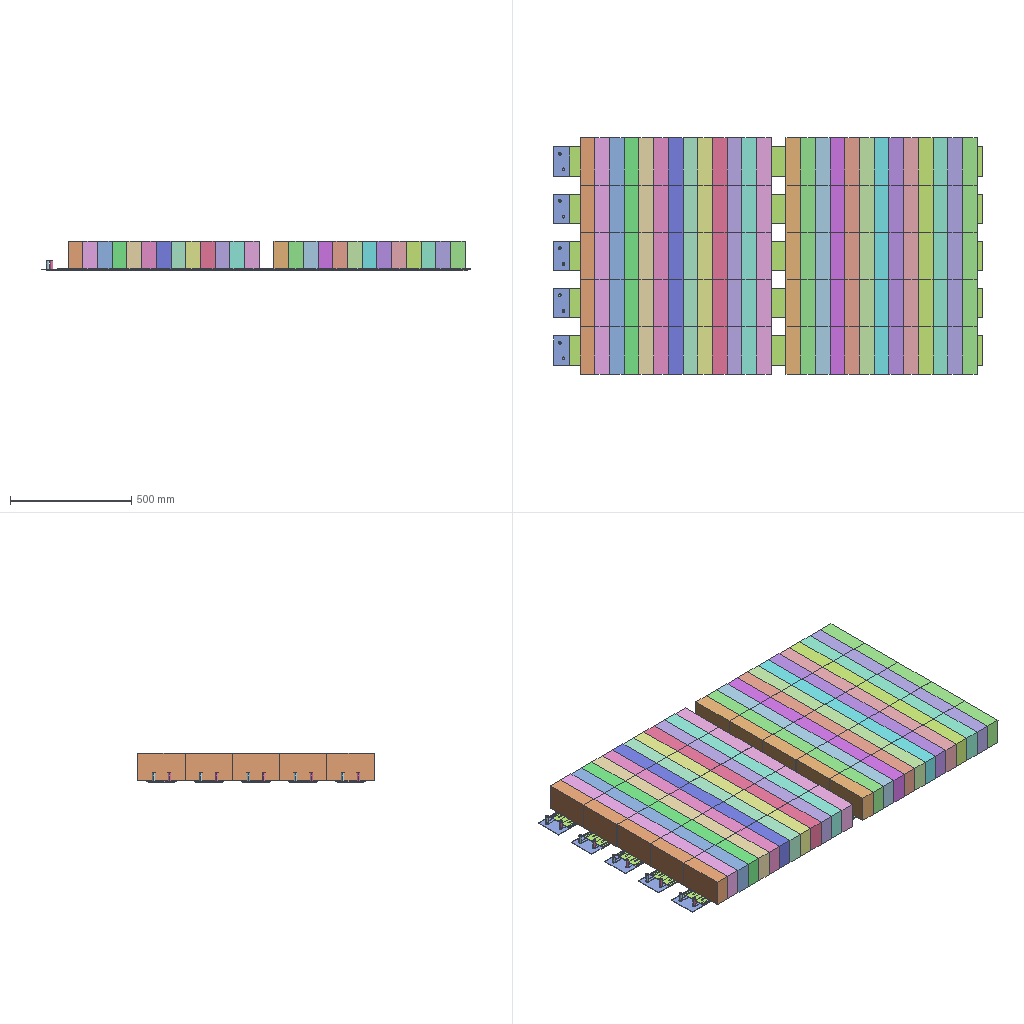Assembly | SolidWorks | 32 different items | 160 placed | box 1768 x 975 x 120 mm
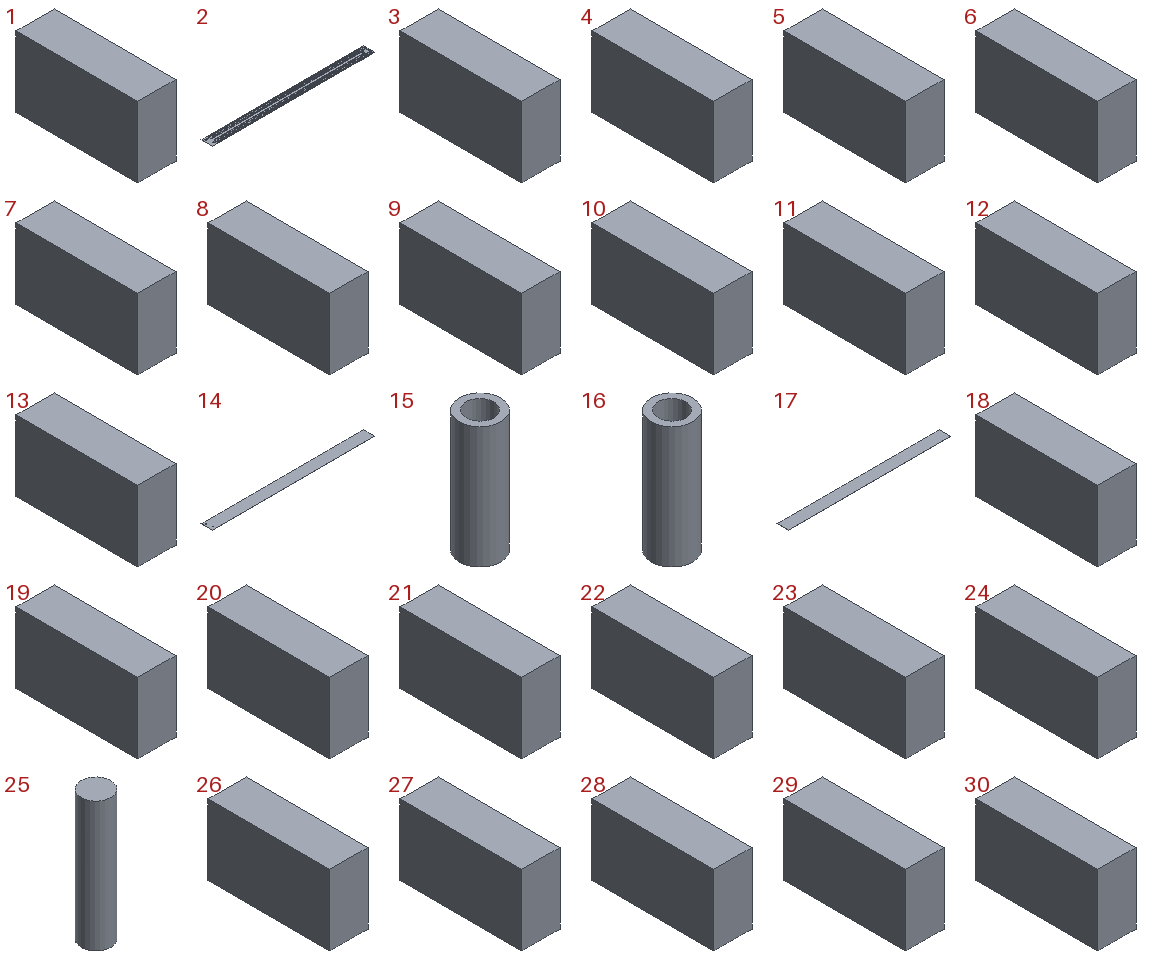Parts list (item | quantity | size | volume | features):
1 | x5 | 60.7 x 194.65 x 112.8 mm | 1332761 mm3 | features BaseBody 1
2 | x5 | 1768 x 120 x 5 mm | 357777 mm3 | features ICE 4, BaseBody 1, LPattern 1
3 | x5 | 60.7 x 194.65 x 112.8 mm | 1332761 mm3 | features BaseBody 1
4 | x5 | 60.7 x 194.65 x 112.8 mm | 1332761 mm3 | features BaseBody 1
5 | x5 | 60.7 x 194.65 x 112.8 mm | 1332761 mm3 | features BaseBody 1
6 | x5 | 60.7 x 194.65 x 112.8 mm | 1332761 mm3 | features BaseBody 1
7 | x5 | 60.7 x 194.65 x 112.8 mm | 1332761 mm3 | features BaseBody 1
8 | x5 | 60.7 x 194.65 x 112.8 mm | 1332761 mm3 | features BaseBody 1
9 | x5 | 60.7 x 194.65 x 112.8 mm | 1332761 mm3 | features BaseBody 1
10 | x5 | 60.7 x 194.65 x 112.8 mm | 1332761 mm3 | features BaseBody 1
11 | x5 | 60.7 x 194.65 x 112.8 mm | 1332761 mm3 | features BaseBody 1
12 | x5 | 60.7 x 194.65 x 112.8 mm | 1332761 mm3 | features BaseBody 1
13 | x5 | 60.7 x 194.65 x 112.8 mm | 1332761 mm3 | features BaseBody 1
14 | x5 | 1768 x 120 x 1 mm | 211934 mm3 | features BaseBody 1
15 | x5 | 12 x 12 x 35 mm | 2199 mm3 | features BaseBody 1
16 | x5 | 12 x 12 x 35 mm | 2199 mm3 | features BaseBody 1
17 | x5 | 1703 x 120 x 1 mm | 204360 mm3 | features BaseBody 1
18 | x5 | 60.7 x 194.65 x 112.8 mm | 1332761 mm3 | features BaseBody 1
19 | x5 | 60.7 x 194.65 x 112.8 mm | 1332761 mm3 | features BaseBody 1
20 | x5 | 60.7 x 194.65 x 112.8 mm | 1332761 mm3 | features BaseBody 1
21 | x5 | 60.7 x 194.65 x 112.8 mm | 1332761 mm3 | features BaseBody 1
22 | x5 | 60.7 x 194.65 x 112.8 mm | 1332761 mm3 | features BaseBody 1
23 | x5 | 60.7 x 194.65 x 112.8 mm | 1332761 mm3 | features BaseBody 1
24 | x5 | 60.7 x 194.65 x 112.8 mm | 1332761 mm3 | features BaseBody 1
25 | x5 | 8 x 8 x 35 mm | 1759 mm3 | features BaseBody 1
26 | x5 | 60.7 x 194.65 x 112.8 mm | 1332761 mm3 | features BaseBody 1
27 | x5 | 60.7 x 194.65 x 112.8 mm | 1332761 mm3 | features BaseBody 1
28 | x5 | 60.7 x 194.65 x 112.8 mm | 1332761 mm3 | features BaseBody 1
29 | x5 | 60.7 x 194.65 x 112.8 mm | 1332761 mm3 | features BaseBody 1
30 | x5 | 60.7 x 194.65 x 112.8 mm | 1332761 mm3 | features BaseBody 1
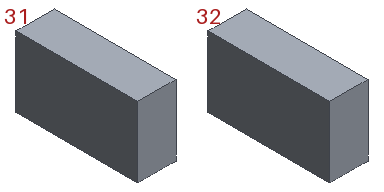31 | x5 | 60.7 x 194.65 x 112.8 mm | 1332761 mm3 | features BaseBody 1
32 | x5 | 60.7 x 194.65 x 112.8 mm | 1332761 mm3 | features BaseBody 1